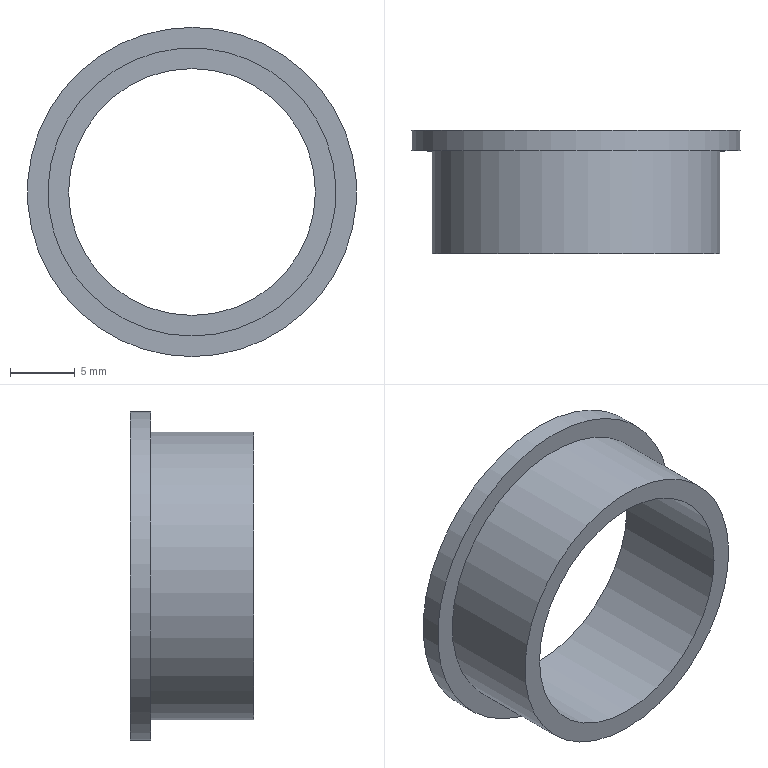Part | NX | features MG0330 trunion parts 24(trunion group) 2 | 1 solid | 6 faces | box 25.4 x 9.525 x 25.4 mm | volume 1170 mm3 | cylinder 3 | plane 3 | commonest cylinder face diameters 19.05 x1 22.228 x1 25.4 x1
STEP:
#1=CARTESIAN_POINT('',(0.,9.779,-11.114));
#2=VERTEX_POINT('',#1);
#3=CARTESIAN_POINT('',(0.,9.779,0.));
#4=DIRECTION('',(0.,-1.,0.));
#5=DIRECTION('',(0.,0.,-1.));
#6=AXIS2_PLACEMENT_3D('',#3,#4,#5);
#7=CIRCLE('',#6,11.114);
#8=EDGE_CURVE('',#2,#2,#7,.T.);
#9=ORIENTED_EDGE('',*,*,#8,.T.);
#10=EDGE_LOOP('',(#9));
#11=FACE_BOUND('',#10,.T.);
#12=CARTESIAN_POINT('',(0.,1.841,-11.114));
#13=VERTEX_POINT('',#12);
#14=CARTESIAN_POINT('',(0.,1.841,0.));
#15=DIRECTION('',(0.,-1.,0.));
#16=DIRECTION('',(0.,0.,-1.));
#17=AXIS2_PLACEMENT_3D('',#14,#15,#16);
#18=CIRCLE('',#17,11.114);
#19=EDGE_CURVE('',#13,#13,#18,.T.);
#20=ORIENTED_EDGE('',*,*,#19,.F.);
#21=EDGE_LOOP('',(#20));
#22=FACE_BOUND('',#21,.T.);
#23=CARTESIAN_POINT('',(0.,0.,0.));
#24=DIRECTION('',(0.,-1.,0.));
#25=DIRECTION('',(0.,0.,-1.));
#26=AXIS2_PLACEMENT_3D('',#23,#24,#25);
#27=CYLINDRICAL_SURFACE('',#26,11.114);
#28=ADVANCED_FACE('',(#11,#22),#27,.T.);
#29=ORIENTED_EDGE('',*,*,#19,.T.);
#30=EDGE_LOOP('',(#29));
#31=FACE_BOUND('',#30,.T.);
#32=CARTESIAN_POINT('',(0.,1.841,-9.525));
#33=VERTEX_POINT('',#32);
#34=CARTESIAN_POINT('',(0.,1.841,0.));
#35=DIRECTION('',(0.,-1.,0.));
#36=DIRECTION('',(0.,0.,-1.));
#37=AXIS2_PLACEMENT_3D('',#34,#35,#36);
#38=CIRCLE('',#37,9.525);
#39=EDGE_CURVE('',#33,#33,#38,.T.);
#40=ORIENTED_EDGE('',*,*,#39,.F.);
#41=EDGE_LOOP('',(#40));
#42=FACE_BOUND('',#41,.T.);
#43=CARTESIAN_POINT('',(9.525,1.841,0.));
#44=DIRECTION('',(0.,-1.,0.));
#45=DIRECTION('',(0.,0.,-1.));
#46=AXIS2_PLACEMENT_3D('',#43,#44,#45);
#47=PLANE('',#46);
#48=ADVANCED_FACE('',(#31,#42),#47,.T.);
#49=ORIENTED_EDGE('',*,*,#39,.T.);
#50=EDGE_LOOP('',(#49));
#51=FACE_BOUND('',#50,.T.);
#52=CARTESIAN_POINT('',(0.,11.367,-9.525));
#53=VERTEX_POINT('',#52);
#54=CARTESIAN_POINT('',(0.,11.367,0.));
#55=DIRECTION('',(0.,-1.,0.));
#56=DIRECTION('',(0.,0.,-1.));
#57=AXIS2_PLACEMENT_3D('',#54,#55,#56);
#58=CIRCLE('',#57,9.525);
#59=EDGE_CURVE('',#53,#53,#58,.T.);
#60=ORIENTED_EDGE('',*,*,#59,.F.);
#61=EDGE_LOOP('',(#60));
#62=FACE_BOUND('',#61,.T.);
#63=CARTESIAN_POINT('',(0.,0.,0.));
#64=DIRECTION('',(0.,-1.,0.));
#65=DIRECTION('',(0.,0.,-1.));
#66=AXIS2_PLACEMENT_3D('',#63,#64,#65);
#67=CYLINDRICAL_SURFACE('',#66,9.525);
#68=ADVANCED_FACE('',(#51,#62),#67,.F.);
#69=ORIENTED_EDGE('',*,*,#59,.T.);
#70=EDGE_LOOP('',(#69));
#71=FACE_BOUND('',#70,.T.);
#72=CARTESIAN_POINT('',(0.,11.367,-12.7));
#73=VERTEX_POINT('',#72);
#74=CARTESIAN_POINT('',(0.,11.367,0.));
#75=DIRECTION('',(0.,-1.,0.));
#76=DIRECTION('',(0.,0.,-1.));
#77=AXIS2_PLACEMENT_3D('',#74,#75,#76);
#78=CIRCLE('',#77,12.7);
#79=EDGE_CURVE('',#73,#73,#78,.T.);
#80=ORIENTED_EDGE('',*,*,#79,.F.);
#81=EDGE_LOOP('',(#80));
#82=FACE_BOUND('',#81,.T.);
#83=CARTESIAN_POINT('',(12.7,11.367,0.));
#84=DIRECTION('',(0.,1.,0.));
#85=DIRECTION('',(0.,0.,1.));
#86=AXIS2_PLACEMENT_3D('',#83,#84,#85);
#87=PLANE('',#86);
#88=ADVANCED_FACE('',(#71,#82),#87,.T.);
#89=ORIENTED_EDGE('',*,*,#79,.T.);
#90=EDGE_LOOP('',(#89));
#91=FACE_BOUND('',#90,.T.);
#92=CARTESIAN_POINT('',(0.,9.779,-12.7));
#93=VERTEX_POINT('',#92);
#94=CARTESIAN_POINT('',(0.,9.779,0.));
#95=DIRECTION('',(0.,-1.,0.));
#96=DIRECTION('',(0.,0.,-1.));
#97=AXIS2_PLACEMENT_3D('',#94,#95,#96);
#98=CIRCLE('',#97,12.7);
#99=EDGE_CURVE('',#93,#93,#98,.T.);
#100=ORIENTED_EDGE('',*,*,#99,.F.);
#101=EDGE_LOOP('',(#100));
#102=FACE_BOUND('',#101,.T.);
#103=CARTESIAN_POINT('',(0.,0.,0.));
#104=DIRECTION('',(0.,-1.,0.));
#105=DIRECTION('',(0.,0.,-1.));
#106=AXIS2_PLACEMENT_3D('',#103,#104,#105);
#107=CYLINDRICAL_SURFACE('',#106,12.7);
#108=ADVANCED_FACE('',(#91,#102),#107,.T.);
#109=ORIENTED_EDGE('',*,*,#99,.T.);
#110=EDGE_LOOP('',(#109));
#111=FACE_BOUND('',#110,.T.);
#112=ORIENTED_EDGE('',*,*,#8,.F.);
#113=EDGE_LOOP('',(#112));
#114=FACE_BOUND('',#113,.T.);
#115=CARTESIAN_POINT('',(12.7,9.779,0.));
#116=DIRECTION('',(0.,-1.,0.));
#117=DIRECTION('',(0.,0.,-1.));
#118=AXIS2_PLACEMENT_3D('',#115,#116,#117);
#119=PLANE('',#118);
#120=ADVANCED_FACE('',(#111,#114),#119,.T.);
#121=CLOSED_SHELL('',(#28,#48,#68,#88,#108,#120));
#122=MANIFOLD_SOLID_BREP('',#121);
#123=(LENGTH_UNIT()NAMED_UNIT(*)SI_UNIT(.MILLI.,.METRE.));
#124=UNCERTAINTY_MEASURE_WITH_UNIT(LENGTH_MEASURE(0.00001),#123,'','');
#125=(NAMED_UNIT(*)PLANE_ANGLE_UNIT()SI_UNIT($,.RADIAN.));
#126=(NAMED_UNIT(*)SI_UNIT($,.STERADIAN.)SOLID_ANGLE_UNIT());
#127=(GEOMETRIC_REPRESENTATION_CONTEXT(3)GLOBAL_UNCERTAINTY_ASSIGNED_CONTEXT((#124))GLOBAL_UNIT_ASSIGNED_CONTEXT((#123,#125,#126))REPRESENTATION_CONTEXT('',''));
#128=ADVANCED_BREP_SHAPE_REPRESENTATION('',(#122),#127);